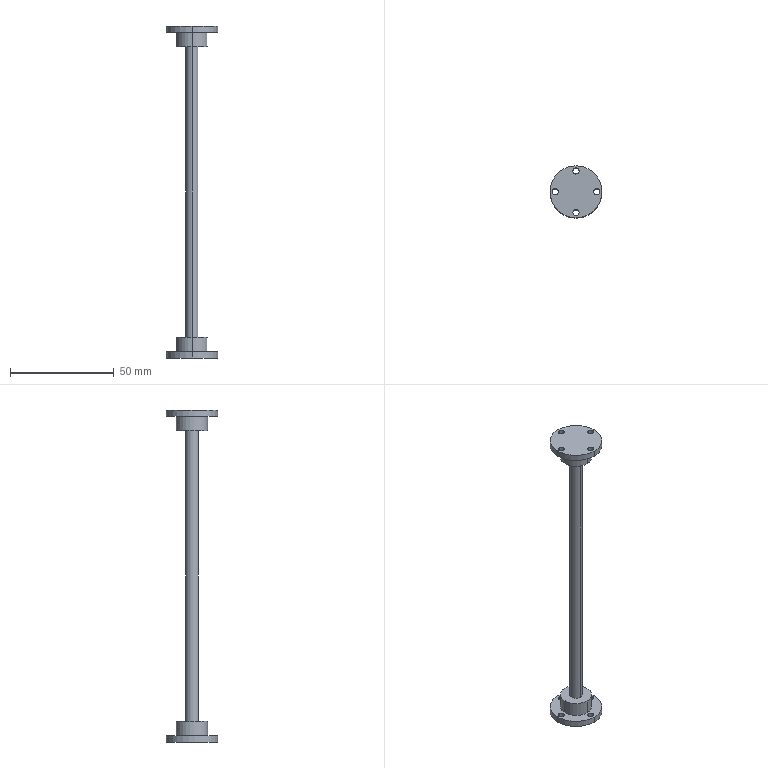Part | SolidWorks | features ICE 1, MirrorPattern 1, Revolution 1 | 1 solid | 32 faces | box 25 x 25 x 160 mm | volume 9208 mm3 | cylinder 26 | plane 6 | commonest cylinder face diameters 3 x16 15 x4 25 x4 6 x2
STEP:
#1=CARTESIAN_POINT('',(-10.,1.5,80.));
#2=VERTEX_POINT('',#1);
#3=CARTESIAN_POINT('',(-10.,-1.5,80.));
#4=VERTEX_POINT('',#3);
#5=CARTESIAN_POINT('',(-10.,0.,80.));
#6=DIRECTION('',(0.,0.,1.));
#7=DIRECTION('',(0.,-1.,0.));
#8=AXIS2_PLACEMENT_3D('',#5,#6,#7);
#9=CIRCLE('',#8,1.5);
#10=EDGE_CURVE('',#2,#4,#9,.T.);
#11=ORIENTED_EDGE('',*,*,#10,.T.);
#12=CARTESIAN_POINT('',(-10.,-1.5,77.));
#13=VERTEX_POINT('',#12);
#14=CARTESIAN_POINT('',(-10.,-1.5,84.));
#15=DIRECTION('',(0.,0.,-1.));
#16=VECTOR('',#15,1000.);
#17=LINE('',#14,#16);
#18=EDGE_CURVE('',#4,#13,#17,.T.);
#19=ORIENTED_EDGE('',*,*,#18,.T.);
#20=CARTESIAN_POINT('',(-10.,1.5,77.));
#21=VERTEX_POINT('',#20);
#22=CARTESIAN_POINT('',(-10.,0.,77.));
#23=DIRECTION('',(0.,0.,-1.));
#24=DIRECTION('',(0.,1.,0.));
#25=AXIS2_PLACEMENT_3D('',#22,#23,#24);
#26=CIRCLE('',#25,1.5);
#27=EDGE_CURVE('',#13,#21,#26,.T.);
#28=ORIENTED_EDGE('',*,*,#27,.T.);
#29=CARTESIAN_POINT('',(-10.,1.5,84.));
#30=DIRECTION('',(0.,0.,-1.));
#31=VECTOR('',#30,1000.);
#32=LINE('',#29,#31);
#33=EDGE_CURVE('',#2,#21,#32,.T.);
#34=ORIENTED_EDGE('',*,*,#33,.F.);
#35=EDGE_LOOP('',(#11,#19,#28,#34));
#36=FACE_OUTER_BOUND('',#35,.T.);
#37=CARTESIAN_POINT('',(-10.,0.,84.));
#38=DIRECTION('',(0.,0.,-1.));
#39=DIRECTION('',(0.,1.,0.));
#40=AXIS2_PLACEMENT_3D('',#37,#38,#39);
#41=CYLINDRICAL_SURFACE('',#40,1.5);
#42=ADVANCED_FACE('',(#36),#41,.F.);
#43=CARTESIAN_POINT('',(0.,-8.5,80.));
#44=VERTEX_POINT('',#43);
#45=CARTESIAN_POINT('',(0.,-11.5,80.));
#46=VERTEX_POINT('',#45);
#47=CARTESIAN_POINT('',(0.,-10.,80.));
#48=DIRECTION('',(0.,0.,1.));
#49=DIRECTION('',(0.,-1.,0.));
#50=AXIS2_PLACEMENT_3D('',#47,#48,#49);
#51=CIRCLE('',#50,1.5);
#52=EDGE_CURVE('',#44,#46,#51,.T.);
#53=ORIENTED_EDGE('',*,*,#52,.T.);
#54=CARTESIAN_POINT('',(0.,-11.5,77.));
#55=VERTEX_POINT('',#54);
#56=CARTESIAN_POINT('',(0.,-11.5,84.));
#57=DIRECTION('',(0.,0.,-1.));
#58=VECTOR('',#57,1000.);
#59=LINE('',#56,#58);
#60=EDGE_CURVE('',#46,#55,#59,.T.);
#61=ORIENTED_EDGE('',*,*,#60,.T.);
#62=CARTESIAN_POINT('',(0.,-8.5,77.));
#63=VERTEX_POINT('',#62);
#64=CARTESIAN_POINT('',(0.,-10.,77.));
#65=DIRECTION('',(0.,0.,-1.));
#66=DIRECTION('',(0.,1.,0.));
#67=AXIS2_PLACEMENT_3D('',#64,#65,#66);
#68=CIRCLE('',#67,1.5);
#69=EDGE_CURVE('',#55,#63,#68,.T.);
#70=ORIENTED_EDGE('',*,*,#69,.T.);
#71=CARTESIAN_POINT('',(0.,-8.5,84.));
#72=DIRECTION('',(0.,0.,-1.));
#73=VECTOR('',#72,1000.);
#74=LINE('',#71,#73);
#75=EDGE_CURVE('',#44,#63,#74,.T.);
#76=ORIENTED_EDGE('',*,*,#75,.F.);
#77=EDGE_LOOP('',(#53,#61,#70,#76));
#78=FACE_OUTER_BOUND('',#77,.T.);
#79=CARTESIAN_POINT('',(0.,-10.,84.));
#80=DIRECTION('',(0.,0.,-1.));
#81=DIRECTION('',(0.,1.,0.));
#82=AXIS2_PLACEMENT_3D('',#79,#80,#81);
#83=CYLINDRICAL_SURFACE('',#82,1.5);
#84=ADVANCED_FACE('',(#78),#83,.F.);
#85=CARTESIAN_POINT('',(10.,1.5,80.));
#86=VERTEX_POINT('',#85);
#87=CARTESIAN_POINT('',(10.,-1.5,80.));
#88=VERTEX_POINT('',#87);
#89=CARTESIAN_POINT('',(10.,0.,80.));
#90=DIRECTION('',(0.,0.,1.));
#91=DIRECTION('',(0.,-1.,0.));
#92=AXIS2_PLACEMENT_3D('',#89,#90,#91);
#93=CIRCLE('',#92,1.5);
#94=EDGE_CURVE('',#86,#88,#93,.T.);
#95=ORIENTED_EDGE('',*,*,#94,.T.);
#96=CARTESIAN_POINT('',(10.,-1.5,77.));
#97=VERTEX_POINT('',#96);
#98=CARTESIAN_POINT('',(10.,-1.5,84.));
#99=DIRECTION('',(0.,0.,-1.));
#100=VECTOR('',#99,1000.);
#101=LINE('',#98,#100);
#102=EDGE_CURVE('',#88,#97,#101,.T.);
#103=ORIENTED_EDGE('',*,*,#102,.T.);
#104=CARTESIAN_POINT('',(10.,1.5,77.));
#105=VERTEX_POINT('',#104);
#106=CARTESIAN_POINT('',(10.,0.,77.));
#107=DIRECTION('',(0.,0.,-1.));
#108=DIRECTION('',(0.,1.,0.));
#109=AXIS2_PLACEMENT_3D('',#106,#107,#108);
#110=CIRCLE('',#109,1.5);
#111=EDGE_CURVE('',#97,#105,#110,.T.);
#112=ORIENTED_EDGE('',*,*,#111,.T.);
#113=CARTESIAN_POINT('',(10.,1.5,84.));
#114=DIRECTION('',(0.,0.,-1.));
#115=VECTOR('',#114,1000.);
#116=LINE('',#113,#115);
#117=EDGE_CURVE('',#86,#105,#116,.T.);
#118=ORIENTED_EDGE('',*,*,#117,.F.);
#119=EDGE_LOOP('',(#95,#103,#112,#118));
#120=FACE_OUTER_BOUND('',#119,.T.);
#121=CARTESIAN_POINT('',(10.,0.,84.));
#122=DIRECTION('',(0.,0.,-1.));
#123=DIRECTION('',(0.,1.,0.));
#124=AXIS2_PLACEMENT_3D('',#121,#122,#123);
#125=CYLINDRICAL_SURFACE('',#124,1.5);
#126=ADVANCED_FACE('',(#120),#125,.F.);
#127=CARTESIAN_POINT('',(0.,11.5,80.));
#128=VERTEX_POINT('',#127);
#129=CARTESIAN_POINT('',(0.,8.5,80.));
#130=VERTEX_POINT('',#129);
#131=CARTESIAN_POINT('',(0.,10.,80.));
#132=DIRECTION('',(0.,0.,1.));
#133=DIRECTION('',(0.,-1.,0.));
#134=AXIS2_PLACEMENT_3D('',#131,#132,#133);
#135=CIRCLE('',#134,1.5);
#136=EDGE_CURVE('',#128,#130,#135,.T.);
#137=ORIENTED_EDGE('',*,*,#136,.T.);
#138=CARTESIAN_POINT('',(0.,8.5,77.));
#139=VERTEX_POINT('',#138);
#140=CARTESIAN_POINT('',(0.,8.5,84.));
#141=DIRECTION('',(0.,0.,-1.));
#142=VECTOR('',#141,1000.);
#143=LINE('',#140,#142);
#144=EDGE_CURVE('',#130,#139,#143,.T.);
#145=ORIENTED_EDGE('',*,*,#144,.T.);
#146=CARTESIAN_POINT('',(0.,11.5,77.));
#147=VERTEX_POINT('',#146);
#148=CARTESIAN_POINT('',(0.,10.,77.));
#149=DIRECTION('',(0.,0.,-1.));
#150=DIRECTION('',(0.,1.,0.));
#151=AXIS2_PLACEMENT_3D('',#148,#149,#150);
#152=CIRCLE('',#151,1.5);
#153=EDGE_CURVE('',#139,#147,#152,.T.);
#154=ORIENTED_EDGE('',*,*,#153,.T.);
#155=CARTESIAN_POINT('',(0.,11.5,84.));
#156=DIRECTION('',(0.,0.,-1.));
#157=VECTOR('',#156,1000.);
#158=LINE('',#155,#157);
#159=EDGE_CURVE('',#128,#147,#158,.T.);
#160=ORIENTED_EDGE('',*,*,#159,.F.);
#161=EDGE_LOOP('',(#137,#145,#154,#160));
#162=FACE_OUTER_BOUND('',#161,.T.);
#163=CARTESIAN_POINT('',(0.,10.,84.));
#164=DIRECTION('',(0.,0.,-1.));
#165=DIRECTION('',(0.,1.,0.));
#166=AXIS2_PLACEMENT_3D('',#163,#164,#165);
#167=CYLINDRICAL_SURFACE('',#166,1.5);
#168=ADVANCED_FACE('',(#162),#167,.F.);
#169=CARTESIAN_POINT('',(-10.,1.5,-77.));
#170=VERTEX_POINT('',#169);
#171=CARTESIAN_POINT('',(-10.,-1.5,-77.));
#172=VERTEX_POINT('',#171);
#173=CARTESIAN_POINT('',(-10.,0.,-77.));
#174=DIRECTION('',(0.,0.,1.));
#175=DIRECTION('',(0.,-1.,0.));
#176=AXIS2_PLACEMENT_3D('',#173,#174,#175);
#177=CIRCLE('',#176,1.5);
#178=EDGE_CURVE('',#170,#172,#177,.T.);
#179=ORIENTED_EDGE('',*,*,#178,.T.);
#180=CARTESIAN_POINT('',(-10.,-1.5,-80.));
#181=VERTEX_POINT('',#180);
#182=CARTESIAN_POINT('',(-10.,-1.5,84.));
#183=DIRECTION('',(0.,0.,-1.));
#184=VECTOR('',#183,1000.);
#185=LINE('',#182,#184);
#186=EDGE_CURVE('',#172,#181,#185,.T.);
#187=ORIENTED_EDGE('',*,*,#186,.T.);
#188=CARTESIAN_POINT('',(-10.,1.5,-80.));
#189=VERTEX_POINT('',#188);
#190=CARTESIAN_POINT('',(-10.,0.,-80.));
#191=DIRECTION('',(0.,0.,-1.));
#192=DIRECTION('',(0.,1.,0.));
#193=AXIS2_PLACEMENT_3D('',#190,#191,#192);
#194=CIRCLE('',#193,1.5);
#195=EDGE_CURVE('',#181,#189,#194,.T.);
#196=ORIENTED_EDGE('',*,*,#195,.T.);
#197=CARTESIAN_POINT('',(-10.,1.5,84.));
#198=DIRECTION('',(0.,0.,-1.));
#199=VECTOR('',#198,1000.);
#200=LINE('',#197,#199);
#201=EDGE_CURVE('',#170,#189,#200,.T.);
#202=ORIENTED_EDGE('',*,*,#201,.F.);
#203=EDGE_LOOP('',(#179,#187,#196,#202));
#204=FACE_OUTER_BOUND('',#203,.T.);
#205=CARTESIAN_POINT('',(-10.,0.,84.));
#206=DIRECTION('',(0.,0.,-1.));
#207=DIRECTION('',(0.,1.,0.));
#208=AXIS2_PLACEMENT_3D('',#205,#206,#207);
#209=CYLINDRICAL_SURFACE('',#208,1.5);
#210=ADVANCED_FACE('',(#204),#209,.F.);
#211=CARTESIAN_POINT('',(0.,-8.5,-77.));
#212=VERTEX_POINT('',#211);
#213=CARTESIAN_POINT('',(0.,-11.5,-77.));
#214=VERTEX_POINT('',#213);
#215=CARTESIAN_POINT('',(0.,-10.,-77.));
#216=DIRECTION('',(0.,0.,1.));
#217=DIRECTION('',(0.,-1.,0.));
#218=AXIS2_PLACEMENT_3D('',#215,#216,#217);
#219=CIRCLE('',#218,1.5);
#220=EDGE_CURVE('',#212,#214,#219,.T.);
#221=ORIENTED_EDGE('',*,*,#220,.T.);
#222=CARTESIAN_POINT('',(0.,-11.5,-80.));
#223=VERTEX_POINT('',#222);
#224=CARTESIAN_POINT('',(0.,-11.5,84.));
#225=DIRECTION('',(0.,0.,-1.));
#226=VECTOR('',#225,1000.);
#227=LINE('',#224,#226);
#228=EDGE_CURVE('',#214,#223,#227,.T.);
#229=ORIENTED_EDGE('',*,*,#228,.T.);
#230=CARTESIAN_POINT('',(0.,-8.5,-80.));
#231=VERTEX_POINT('',#230);
#232=CARTESIAN_POINT('',(0.,-10.,-80.));
#233=DIRECTION('',(0.,0.,-1.));
#234=DIRECTION('',(0.,1.,0.));
#235=AXIS2_PLACEMENT_3D('',#232,#233,#234);
#236=CIRCLE('',#235,1.5);
#237=EDGE_CURVE('',#223,#231,#236,.T.);
#238=ORIENTED_EDGE('',*,*,#237,.T.);
#239=CARTESIAN_POINT('',(0.,-8.5,84.));
#240=DIRECTION('',(0.,0.,-1.));
#241=VECTOR('',#240,1000.);
#242=LINE('',#239,#241);
#243=EDGE_CURVE('',#212,#231,#242,.T.);
#244=ORIENTED_EDGE('',*,*,#243,.F.);
#245=EDGE_LOOP('',(#221,#229,#238,#244));
#246=FACE_OUTER_BOUND('',#245,.T.);
#247=CARTESIAN_POINT('',(0.,-10.,84.));
#248=DIRECTION('',(0.,0.,-1.));
#249=DIRECTION('',(0.,1.,0.));
#250=AXIS2_PLACEMENT_3D('',#247,#248,#249);
#251=CYLINDRICAL_SURFACE('',#250,1.5);
#252=ADVANCED_FACE('',(#246),#251,.F.);
#253=CARTESIAN_POINT('',(10.,1.5,-77.));
#254=VERTEX_POINT('',#253);
#255=CARTESIAN_POINT('',(10.,-1.5,-77.));
#256=VERTEX_POINT('',#255);
#257=CARTESIAN_POINT('',(10.,0.,-77.));
#258=DIRECTION('',(0.,0.,1.));
#259=DIRECTION('',(0.,-1.,0.));
#260=AXIS2_PLACEMENT_3D('',#257,#258,#259);
#261=CIRCLE('',#260,1.5);
#262=EDGE_CURVE('',#254,#256,#261,.T.);
#263=ORIENTED_EDGE('',*,*,#262,.T.);
#264=CARTESIAN_POINT('',(10.,-1.5,-80.));
#265=VERTEX_POINT('',#264);
#266=CARTESIAN_POINT('',(10.,-1.5,84.));
#267=DIRECTION('',(0.,0.,-1.));
#268=VECTOR('',#267,1000.);
#269=LINE('',#266,#268);
#270=EDGE_CURVE('',#256,#265,#269,.T.);
#271=ORIENTED_EDGE('',*,*,#270,.T.);
#272=CARTESIAN_POINT('',(10.,1.5,-80.));
#273=VERTEX_POINT('',#272);
#274=CARTESIAN_POINT('',(10.,0.,-80.));
#275=DIRECTION('',(0.,0.,-1.));
#276=DIRECTION('',(0.,1.,0.));
#277=AXIS2_PLACEMENT_3D('',#274,#275,#276);
#278=CIRCLE('',#277,1.5);
#279=EDGE_CURVE('',#265,#273,#278,.T.);
#280=ORIENTED_EDGE('',*,*,#279,.T.);
#281=CARTESIAN_POINT('',(10.,1.5,84.));
#282=DIRECTION('',(0.,0.,-1.));
#283=VECTOR('',#282,1000.);
#284=LINE('',#281,#283);
#285=EDGE_CURVE('',#254,#273,#284,.T.);
#286=ORIENTED_EDGE('',*,*,#285,.F.);
#287=EDGE_LOOP('',(#263,#271,#280,#286));
#288=FACE_OUTER_BOUND('',#287,.T.);
#289=CARTESIAN_POINT('',(10.,0.,84.));
#290=DIRECTION('',(0.,0.,-1.));
#291=DIRECTION('',(0.,1.,0.));
#292=AXIS2_PLACEMENT_3D('',#289,#290,#291);
#293=CYLINDRICAL_SURFACE('',#292,1.5);
#294=ADVANCED_FACE('',(#288),#293,.F.);
#295=CARTESIAN_POINT('',(0.,11.5,-77.));
#296=VERTEX_POINT('',#295);
#297=CARTESIAN_POINT('',(0.,8.5,-77.));
#298=VERTEX_POINT('',#297);
#299=CARTESIAN_POINT('',(0.,10.,-77.));
#300=DIRECTION('',(0.,0.,1.));
#301=DIRECTION('',(0.,-1.,0.));
#302=AXIS2_PLACEMENT_3D('',#299,#300,#301);
#303=CIRCLE('',#302,1.5);
#304=EDGE_CURVE('',#296,#298,#303,.T.);
#305=ORIENTED_EDGE('',*,*,#304,.T.);
#306=CARTESIAN_POINT('',(0.,8.5,-80.));
#307=VERTEX_POINT('',#306);
#308=CARTESIAN_POINT('',(0.,8.5,84.));
#309=DIRECTION('',(0.,0.,-1.));
#310=VECTOR('',#309,1000.);
#311=LINE('',#308,#310);
#312=EDGE_CURVE('',#298,#307,#311,.T.);
#313=ORIENTED_EDGE('',*,*,#312,.T.);
#314=CARTESIAN_POINT('',(0.,11.5,-80.));
#315=VERTEX_POINT('',#314);
#316=CARTESIAN_POINT('',(0.,10.,-80.));
#317=DIRECTION('',(0.,0.,-1.));
#318=DIRECTION('',(0.,1.,0.));
#319=AXIS2_PLACEMENT_3D('',#316,#317,#318);
#320=CIRCLE('',#319,1.5);
#321=EDGE_CURVE('',#307,#315,#320,.T.);
#322=ORIENTED_EDGE('',*,*,#321,.T.);
#323=CARTESIAN_POINT('',(0.,11.5,84.));
#324=DIRECTION('',(0.,0.,-1.));
#325=VECTOR('',#324,1000.);
#326=LINE('',#323,#325);
#327=EDGE_CURVE('',#296,#315,#326,.T.);
#328=ORIENTED_EDGE('',*,*,#327,.F.);
#329=EDGE_LOOP('',(#305,#313,#322,#328));
#330=FACE_OUTER_BOUND('',#329,.T.);
#331=CARTESIAN_POINT('',(0.,10.,84.));
#332=DIRECTION('',(0.,0.,-1.));
#333=DIRECTION('',(0.,1.,0.));
#334=AXIS2_PLACEMENT_3D('',#331,#332,#333);
#335=CYLINDRICAL_SURFACE('',#334,1.5);
#336=ADVANCED_FACE('',(#330),#335,.F.);
#337=CARTESIAN_POINT('',(0.,-7.5,-77.));
#338=VERTEX_POINT('',#337);
#339=CARTESIAN_POINT('',(0.,7.5,-77.));
#340=VERTEX_POINT('',#339);
#341=CARTESIAN_POINT('',(0.,0.,-77.));
#342=DIRECTION('',(0.,0.,-1.));
#343=DIRECTION('',(0.,1.,0.));
#344=AXIS2_PLACEMENT_3D('',#341,#342,#343);
#345=CIRCLE('',#344,7.5);
#346=EDGE_CURVE('',#338,#340,#345,.T.);
#347=ORIENTED_EDGE('',*,*,#346,.F.);
#348=CARTESIAN_POINT('',(0.,-7.5,-70.));
#349=VERTEX_POINT('',#348);
#350=CARTESIAN_POINT('',(0.,-7.5,0.));
#351=DIRECTION('',(0.,0.,1.));
#352=VECTOR('',#351,1000.);
#353=LINE('',#350,#352);
#354=EDGE_CURVE('',#338,#349,#353,.T.);
#355=ORIENTED_EDGE('',*,*,#354,.T.);
#356=CARTESIAN_POINT('',(0.,7.5,-70.));
#357=VERTEX_POINT('',#356);
#358=CARTESIAN_POINT('',(0.,0.,-70.));
#359=DIRECTION('',(0.,0.,-1.));
#360=DIRECTION('',(0.,1.,0.));
#361=AXIS2_PLACEMENT_3D('',#358,#359,#360);
#362=CIRCLE('',#361,7.5);
#363=EDGE_CURVE('',#349,#357,#362,.T.);
#364=ORIENTED_EDGE('',*,*,#363,.T.);
#365=CARTESIAN_POINT('',(0.,7.5,0.));
#366=DIRECTION('',(0.,0.,1.));
#367=VECTOR('',#366,1000.);
#368=LINE('',#365,#367);
#369=EDGE_CURVE('',#340,#357,#368,.T.);
#370=ORIENTED_EDGE('',*,*,#369,.F.);
#371=EDGE_LOOP('',(#347,#355,#364,#370));
#372=FACE_OUTER_BOUND('',#371,.T.);
#373=CARTESIAN_POINT('',(0.,0.,0.));
#374=DIRECTION('',(0.,0.,1.));
#375=DIRECTION('',(0.,1.,0.));
#376=AXIS2_PLACEMENT_3D('',#373,#374,#375);
#377=CYLINDRICAL_SURFACE('',#376,7.5);
#378=ADVANCED_FACE('',(#372),#377,.T.);
#379=CARTESIAN_POINT('',(0.,-12.5,-80.));
#380=VERTEX_POINT('',#379);
#381=CARTESIAN_POINT('',(0.,12.5,-80.));
#382=VERTEX_POINT('',#381);
#383=CARTESIAN_POINT('',(0.,0.,-80.));
#384=DIRECTION('',(0.,0.,-1.));
#385=DIRECTION('',(0.,1.,0.));
#386=AXIS2_PLACEMENT_3D('',#383,#384,#385);
#387=CIRCLE('',#386,12.5);
#388=EDGE_CURVE('',#380,#382,#387,.T.);
#389=ORIENTED_EDGE('',*,*,#388,.F.);
#390=CARTESIAN_POINT('',(0.,-12.5,-77.));
#391=VERTEX_POINT('',#390);
#392=CARTESIAN_POINT('',(0.,-12.5,0.));
#393=DIRECTION('',(0.,0.,1.));
#394=VECTOR('',#393,1000.);
#395=LINE('',#392,#394);
#396=EDGE_CURVE('',#380,#391,#395,.T.);
#397=ORIENTED_EDGE('',*,*,#396,.T.);
#398=CARTESIAN_POINT('',(0.,12.5,-77.));
#399=VERTEX_POINT('',#398);
#400=CARTESIAN_POINT('',(0.,0.,-77.));
#401=DIRECTION('',(0.,0.,-1.));
#402=DIRECTION('',(0.,1.,0.));
#403=AXIS2_PLACEMENT_3D('',#400,#401,#402);
#404=CIRCLE('',#403,12.5);
#405=EDGE_CURVE('',#391,#399,#404,.T.);
#406=ORIENTED_EDGE('',*,*,#405,.T.);
#407=CARTESIAN_POINT('',(0.,12.5,0.));
#408=DIRECTION('',(0.,0.,1.));
#409=VECTOR('',#408,1000.);
#410=LINE('',#407,#409);
#411=EDGE_CURVE('',#382,#399,#410,.T.);
#412=ORIENTED_EDGE('',*,*,#411,.F.);
#413=EDGE_LOOP('',(#389,#397,#406,#412));
#414=FACE_OUTER_BOUND('',#413,.T.);
#415=CARTESIAN_POINT('',(0.,0.,0.));
#416=DIRECTION('',(0.,0.,1.));
#417=DIRECTION('',(0.,1.,0.));
#418=AXIS2_PLACEMENT_3D('',#415,#416,#417);
#419=CYLINDRICAL_SURFACE('',#418,12.5);
#420=ADVANCED_FACE('',(#414),#419,.T.);
#421=CARTESIAN_POINT('',(0.,3.,70.));
#422=VERTEX_POINT('',#421);
#423=CARTESIAN_POINT('',(0.,-3.,70.));
#424=VERTEX_POINT('',#423);
#425=CARTESIAN_POINT('',(0.,0.,70.));
#426=DIRECTION('',(0.,0.,-1.));
#427=DIRECTION('',(0.,1.,0.));
#428=AXIS2_PLACEMENT_3D('',#425,#426,#427);
#429=CIRCLE('',#428,3.);
#430=EDGE_CURVE('',#422,#424,#429,.T.);
#431=ORIENTED_EDGE('',*,*,#430,.T.);
#432=CARTESIAN_POINT('',(0.,-3.,-70.));
#433=VERTEX_POINT('',#432);
#434=CARTESIAN_POINT('',(0.,-3.,0.));
#435=DIRECTION('',(0.,0.,-1.));
#436=VECTOR('',#435,1000.);
#437=LINE('',#434,#436);
#438=EDGE_CURVE('',#424,#433,#437,.T.);
#439=ORIENTED_EDGE('',*,*,#438,.T.);
#440=CARTESIAN_POINT('',(0.,3.,-70.));
#441=VERTEX_POINT('',#440);
#442=CARTESIAN_POINT('',(0.,0.,-70.));
#443=DIRECTION('',(0.,0.,-1.));
#444=DIRECTION('',(0.,1.,0.));
#445=AXIS2_PLACEMENT_3D('',#442,#443,#444);
#446=CIRCLE('',#445,3.);
#447=EDGE_CURVE('',#441,#433,#446,.T.);
#448=ORIENTED_EDGE('',*,*,#447,.F.);
#449=CARTESIAN_POINT('',(0.,3.,0.));
#450=DIRECTION('',(0.,0.,-1.));
#451=VECTOR('',#450,1000.);
#452=LINE('',#449,#451);
#453=EDGE_CURVE('',#422,#441,#452,.T.);
#454=ORIENTED_EDGE('',*,*,#453,.F.);
#455=EDGE_LOOP('',(#431,#439,#448,#454));
#456=FACE_OUTER_BOUND('',#455,.T.);
#457=CARTESIAN_POINT('',(0.,0.,0.));
#458=DIRECTION('',(0.,0.,-1.));
#459=DIRECTION('',(0.,1.,0.));
#460=AXIS2_PLACEMENT_3D('',#457,#458,#459);
#461=CYLINDRICAL_SURFACE('',#460,3.);
#462=ADVANCED_FACE('',(#456),#461,.T.);
#463=CARTESIAN_POINT('',(0.,7.5,77.));
#464=VERTEX_POINT('',#463);
#465=CARTESIAN_POINT('',(0.,-7.5,77.));
#466=VERTEX_POINT('',#465);
#467=CARTESIAN_POINT('',(0.,0.,77.));
#468=DIRECTION('',(0.,0.,-1.));
#469=DIRECTION('',(0.,1.,0.));
#470=AXIS2_PLACEMENT_3D('',#467,#468,#469);
#471=CIRCLE('',#470,7.5);
#472=EDGE_CURVE('',#464,#466,#471,.T.);
#473=ORIENTED_EDGE('',*,*,#472,.T.);
#474=CARTESIAN_POINT('',(0.,-7.5,70.));
#475=VERTEX_POINT('',#474);
#476=CARTESIAN_POINT('',(0.,-7.5,0.));
#477=DIRECTION('',(0.,0.,-1.));
#478=VECTOR('',#477,1000.);
#479=LINE('',#476,#478);
#480=EDGE_CURVE('',#466,#475,#479,.T.);
#481=ORIENTED_EDGE('',*,*,#480,.T.);
#482=CARTESIAN_POINT('',(0.,7.5,70.));
#483=VERTEX_POINT('',#482);
#484=CARTESIAN_POINT('',(0.,0.,70.));
#485=DIRECTION('',(0.,0.,-1.));
#486=DIRECTION('',(0.,1.,0.));
#487=AXIS2_PLACEMENT_3D('',#484,#485,#486);
#488=CIRCLE('',#487,7.5);
#489=EDGE_CURVE('',#483,#475,#488,.T.);
#490=ORIENTED_EDGE('',*,*,#489,.F.);
#491=CARTESIAN_POINT('',(0.,7.5,0.));
#492=DIRECTION('',(0.,0.,-1.));
#493=VECTOR('',#492,1000.);
#494=LINE('',#491,#493);
#495=EDGE_CURVE('',#464,#483,#494,.T.);
#496=ORIENTED_EDGE('',*,*,#495,.F.);
#497=EDGE_LOOP('',(#473,#481,#490,#496));
#498=FACE_OUTER_BOUND('',#497,.T.);
#499=CARTESIAN_POINT('',(0.,0.,0.));
#500=DIRECTION('',(0.,0.,-1.));
#501=DIRECTION('',(0.,1.,0.));
#502=AXIS2_PLACEMENT_3D('',#499,#500,#501);
#503=CYLINDRICAL_SURFACE('',#502,7.5);
#504=ADVANCED_FACE('',(#498),#503,.T.);
#505=CARTESIAN_POINT('',(0.,12.5,80.));
#506=VERTEX_POINT('',#505);
#507=CARTESIAN_POINT('',(0.,-12.5,80.));
#508=VERTEX_POINT('',#507);
#509=CARTESIAN_POINT('',(0.,0.,80.));
#510=DIRECTION('',(0.,0.,-1.));
#511=DIRECTION('',(0.,1.,0.));
#512=AXIS2_PLACEMENT_3D('',#509,#510,#511);
#513=CIRCLE('',#512,12.5);
#514=EDGE_CURVE('',#506,#508,#513,.T.);
#515=ORIENTED_EDGE('',*,*,#514,.T.);
#516=CARTESIAN_POINT('',(0.,-12.5,77.));
#517=VERTEX_POINT('',#516);
#518=CARTESIAN_POINT('',(0.,-12.5,0.));
#519=DIRECTION('',(0.,0.,-1.));
#520=VECTOR('',#519,1000.);
#521=LINE('',#518,#520);
#522=EDGE_CURVE('',#508,#517,#521,.T.);
#523=ORIENTED_EDGE('',*,*,#522,.T.);
#524=CARTESIAN_POINT('',(0.,12.5,77.));
#525=VERTEX_POINT('',#524);
#526=CARTESIAN_POINT('',(0.,0.,77.));
#527=DIRECTION('',(0.,0.,-1.));
#528=DIRECTION('',(0.,1.,0.));
#529=AXIS2_PLACEMENT_3D('',#526,#527,#528);
#530=CIRCLE('',#529,12.5);
#531=EDGE_CURVE('',#525,#517,#530,.T.);
#532=ORIENTED_EDGE('',*,*,#531,.F.);
#533=CARTESIAN_POINT('',(0.,12.5,0.));
#534=DIRECTION('',(0.,0.,-1.));
#535=VECTOR('',#534,1000.);
#536=LINE('',#533,#535);
#537=EDGE_CURVE('',#506,#525,#536,.T.);
#538=ORIENTED_EDGE('',*,*,#537,.F.);
#539=EDGE_LOOP('',(#515,#523,#532,#538));
#540=FACE_OUTER_BOUND('',#539,.T.);
#541=CARTESIAN_POINT('',(0.,0.,0.));
#542=DIRECTION('',(0.,0.,-1.));
#543=DIRECTION('',(0.,1.,0.));
#544=AXIS2_PLACEMENT_3D('',#541,#542,#543);
#545=CYLINDRICAL_SURFACE('',#544,12.5);
#546=ADVANCED_FACE('',(#540),#545,.T.);
#547=ORIENTED_EDGE('',*,*,#10,.F.);
#548=CARTESIAN_POINT('',(-10.,0.,80.));
#549=DIRECTION('',(0.,0.,1.));
#550=DIRECTION('',(0.,-1.,0.));
#551=AXIS2_PLACEMENT_3D('',#548,#549,#550);
#552=CIRCLE('',#551,1.5);
#553=EDGE_CURVE('',#4,#2,#552,.T.);
#554=ORIENTED_EDGE('',*,*,#553,.F.);
#555=EDGE_LOOP('',(#547,#554));
#556=FACE_BOUND('',#555,.T.);
#557=ORIENTED_EDGE('',*,*,#52,.F.);
#558=CARTESIAN_POINT('',(0.,-10.,80.));
#559=DIRECTION('',(0.,0.,1.));
#560=DIRECTION('',(0.,-1.,0.));
#561=AXIS2_PLACEMENT_3D('',#558,#559,#560);
#562=CIRCLE('',#561,1.5);
#563=EDGE_CURVE('',#46,#44,#562,.T.);
#564=ORIENTED_EDGE('',*,*,#563,.F.);
#565=EDGE_LOOP('',(#557,#564));
#566=FACE_BOUND('',#565,.T.);
#567=ORIENTED_EDGE('',*,*,#94,.F.);
#568=CARTESIAN_POINT('',(10.,0.,80.));
#569=DIRECTION('',(0.,0.,1.));
#570=DIRECTION('',(0.,-1.,0.));
#571=AXIS2_PLACEMENT_3D('',#568,#569,#570);
#572=CIRCLE('',#571,1.5);
#573=EDGE_CURVE('',#88,#86,#572,.T.);
#574=ORIENTED_EDGE('',*,*,#573,.F.);
#575=EDGE_LOOP('',(#567,#574));
#576=FACE_BOUND('',#575,.T.);
#577=ORIENTED_EDGE('',*,*,#136,.F.);
#578=CARTESIAN_POINT('',(0.,10.,80.));
#579=DIRECTION('',(0.,0.,1.));
#580=DIRECTION('',(0.,-1.,0.));
#581=AXIS2_PLACEMENT_3D('',#578,#579,#580);
#582=CIRCLE('',#581,1.5);
#583=EDGE_CURVE('',#130,#128,#582,.T.);
#584=ORIENTED_EDGE('',*,*,#583,.F.);
#585=EDGE_LOOP('',(#577,#584));
#586=FACE_BOUND('',#585,.T.);
#587=ORIENTED_EDGE('',*,*,#514,.F.);
#588=CARTESIAN_POINT('',(0.,0.,80.));
#589=DIRECTION('',(0.,0.,-1.));
#590=DIRECTION('',(0.,1.,0.));
#591=AXIS2_PLACEMENT_3D('',#588,#589,#590);
#592=CIRCLE('',#591,12.5);
#593=EDGE_CURVE('',#508,#506,#592,.T.);
#594=ORIENTED_EDGE('',*,*,#593,.F.);
#595=EDGE_LOOP('',(#587,#594));
#596=FACE_OUTER_BOUND('',#595,.T.);
#597=CARTESIAN_POINT('',(0.,0.,80.));
#598=DIRECTION('',(0.,0.,1.));
#599=DIRECTION('',(0.,-1.,0.));
#600=AXIS2_PLACEMENT_3D('',#597,#598,#599);
#601=PLANE('',#600);
#602=ADVANCED_FACE('',(#556,#566,#576,#586,#596),#601,.T.);
#603=ORIENTED_EDGE('',*,*,#522,.F.);
#604=ORIENTED_EDGE('',*,*,#593,.T.);
#605=ORIENTED_EDGE('',*,*,#537,.T.);
#606=CARTESIAN_POINT('',(0.,0.,77.));
#607=DIRECTION('',(0.,0.,-1.));
#608=DIRECTION('',(0.,1.,0.));
#609=AXIS2_PLACEMENT_3D('',#606,#607,#608);
#610=CIRCLE('',#609,12.5);
#611=EDGE_CURVE('',#517,#525,#610,.T.);
#612=ORIENTED_EDGE('',*,*,#611,.F.);
#613=EDGE_LOOP('',(#603,#604,#605,#612));
#614=FACE_OUTER_BOUND('',#613,.T.);
#615=CARTESIAN_POINT('',(0.,0.,0.));
#616=DIRECTION('',(0.,0.,-1.));
#617=DIRECTION('',(0.,1.,0.));
#618=AXIS2_PLACEMENT_3D('',#615,#616,#617);
#619=CYLINDRICAL_SURFACE('',#618,12.5);
#620=ADVANCED_FACE('',(#614),#619,.T.);
#621=CARTESIAN_POINT('',(-10.,0.,77.));
#622=DIRECTION('',(0.,0.,-1.));
#623=DIRECTION('',(0.,1.,0.));
#624=AXIS2_PLACEMENT_3D('',#621,#622,#623);
#625=CIRCLE('',#624,1.5);
#626=EDGE_CURVE('',#21,#13,#625,.T.);
#627=ORIENTED_EDGE('',*,*,#626,.F.);
#628=ORIENTED_EDGE('',*,*,#27,.F.);
#629=EDGE_LOOP('',(#627,#628));
#630=FACE_BOUND('',#629,.T.);
#631=CARTESIAN_POINT('',(0.,-10.,77.));
#632=DIRECTION('',(0.,0.,-1.));
#633=DIRECTION('',(0.,1.,0.));
#634=AXIS2_PLACEMENT_3D('',#631,#632,#633);
#635=CIRCLE('',#634,1.5);
#636=EDGE_CURVE('',#63,#55,#635,.T.);
#637=ORIENTED_EDGE('',*,*,#636,.F.);
#638=ORIENTED_EDGE('',*,*,#69,.F.);
#639=EDGE_LOOP('',(#637,#638));
#640=FACE_BOUND('',#639,.T.);
#641=CARTESIAN_POINT('',(10.,0.,77.));
#642=DIRECTION('',(0.,0.,-1.));
#643=DIRECTION('',(0.,1.,0.));
#644=AXIS2_PLACEMENT_3D('',#641,#642,#643);
#645=CIRCLE('',#644,1.5);
#646=EDGE_CURVE('',#105,#97,#645,.T.);
#647=ORIENTED_EDGE('',*,*,#646,.F.);
#648=ORIENTED_EDGE('',*,*,#111,.F.);
#649=EDGE_LOOP('',(#647,#648));
#650=FACE_BOUND('',#649,.T.);
#651=CARTESIAN_POINT('',(0.,10.,77.));
#652=DIRECTION('',(0.,0.,-1.));
#653=DIRECTION('',(0.,1.,0.));
#654=AXIS2_PLACEMENT_3D('',#651,#652,#653);
#655=CIRCLE('',#654,1.5);
#656=EDGE_CURVE('',#147,#139,#655,.T.);
#657=ORIENTED_EDGE('',*,*,#656,.F.);
#658=ORIENTED_EDGE('',*,*,#153,.F.);
#659=EDGE_LOOP('',(#657,#658));
#660=FACE_BOUND('',#659,.T.);
#661=ORIENTED_EDGE('',*,*,#531,.T.);
#662=ORIENTED_EDGE('',*,*,#611,.T.);
#663=EDGE_LOOP('',(#661,#662));
#664=FACE_OUTER_BOUND('',#663,.T.);
#665=ORIENTED_EDGE('',*,*,#472,.F.);
#666=CARTESIAN_POINT('',(0.,0.,77.));
#667=DIRECTION('',(0.,0.,-1.));
#668=DIRECTION('',(0.,1.,0.));
#669=AXIS2_PLACEMENT_3D('',#666,#667,#668);
#670=CIRCLE('',#669,7.5);
#671=EDGE_CURVE('',#466,#464,#670,.T.);
#672=ORIENTED_EDGE('',*,*,#671,.F.);
#673=EDGE_LOOP('',(#665,#672));
#674=FACE_BOUND('',#673,.T.);
#675=CARTESIAN_POINT('',(0.,12.5,77.));
#676=DIRECTION('',(0.,0.,-1.));
#677=DIRECTION('',(0.,1.,0.));
#678=AXIS2_PLACEMENT_3D('',#675,#676,#677);
#679=PLANE('',#678);
#680=ADVANCED_FACE('',(#630,#640,#650,#660,#664,#674),#679,.T.);
#681=ORIENTED_EDGE('',*,*,#480,.F.);
#682=ORIENTED_EDGE('',*,*,#671,.T.);
#683=ORIENTED_EDGE('',*,*,#495,.T.);
#684=CARTESIAN_POINT('',(0.,0.,70.));
#685=DIRECTION('',(0.,0.,-1.));
#686=DIRECTION('',(0.,1.,0.));
#687=AXIS2_PLACEMENT_3D('',#684,#685,#686);
#688=CIRCLE('',#687,7.5);
#689=EDGE_CURVE('',#475,#483,#688,.T.);
#690=ORIENTED_EDGE('',*,*,#689,.F.);
#691=EDGE_LOOP('',(#681,#682,#683,#690));
#692=FACE_OUTER_BOUND('',#691,.T.);
#693=CARTESIAN_POINT('',(0.,0.,0.));
#694=DIRECTION('',(0.,0.,-1.));
#695=DIRECTION('',(0.,1.,0.));
#696=AXIS2_PLACEMENT_3D('',#693,#694,#695);
#697=CYLINDRICAL_SURFACE('',#696,7.5);
#698=ADVANCED_FACE('',(#692),#697,.T.);
#699=ORIENTED_EDGE('',*,*,#489,.T.);
#700=ORIENTED_EDGE('',*,*,#689,.T.);
#701=EDGE_LOOP('',(#699,#700));
#702=FACE_OUTER_BOUND('',#701,.T.);
#703=ORIENTED_EDGE('',*,*,#430,.F.);
#704=CARTESIAN_POINT('',(0.,0.,70.));
#705=DIRECTION('',(0.,0.,-1.));
#706=DIRECTION('',(0.,1.,0.));
#707=AXIS2_PLACEMENT_3D('',#704,#705,#706);
#708=CIRCLE('',#707,3.);
#709=EDGE_CURVE('',#424,#422,#708,.T.);
#710=ORIENTED_EDGE('',*,*,#709,.F.);
#711=EDGE_LOOP('',(#703,#710));
#712=FACE_BOUND('',#711,.T.);
#713=CARTESIAN_POINT('',(0.,7.5,70.));
#714=DIRECTION('',(0.,0.,-1.));
#715=DIRECTION('',(0.,1.,0.));
#716=AXIS2_PLACEMENT_3D('',#713,#714,#715);
#717=PLANE('',#716);
#718=ADVANCED_FACE('',(#702,#712),#717,.T.);
#719=ORIENTED_EDGE('',*,*,#438,.F.);
#720=ORIENTED_EDGE('',*,*,#709,.T.);
#721=ORIENTED_EDGE('',*,*,#453,.T.);
#722=CARTESIAN_POINT('',(0.,0.,-70.));
#723=DIRECTION('',(0.,0.,-1.));
#724=DIRECTION('',(0.,1.,0.));
#725=AXIS2_PLACEMENT_3D('',#722,#723,#724);
#726=CIRCLE('',#725,3.);
#727=EDGE_CURVE('',#433,#441,#726,.T.);
#728=ORIENTED_EDGE('',*,*,#727,.F.);
#729=EDGE_LOOP('',(#719,#720,#721,#728));
#730=FACE_OUTER_BOUND('',#729,.T.);
#731=CARTESIAN_POINT('',(0.,0.,0.));
#732=DIRECTION('',(0.,0.,-1.));
#733=DIRECTION('',(0.,1.,0.));
#734=AXIS2_PLACEMENT_3D('',#731,#732,#733);
#735=CYLINDRICAL_SURFACE('',#734,3.);
#736=ADVANCED_FACE('',(#730),#735,.T.);
#737=CARTESIAN_POINT('',(-10.,0.,-80.));
#738=DIRECTION('',(0.,0.,-1.));
#739=DIRECTION('',(0.,1.,0.));
#740=AXIS2_PLACEMENT_3D('',#737,#738,#739);
#741=CIRCLE('',#740,1.5);
#742=EDGE_CURVE('',#189,#181,#741,.T.);
#743=ORIENTED_EDGE('',*,*,#742,.F.);
#744=ORIENTED_EDGE('',*,*,#195,.F.);
#745=EDGE_LOOP('',(#743,#744));
#746=FACE_BOUND('',#745,.T.);
#747=CARTESIAN_POINT('',(0.,-10.,-80.));
#748=DIRECTION('',(0.,0.,-1.));
#749=DIRECTION('',(0.,1.,0.));
#750=AXIS2_PLACEMENT_3D('',#747,#748,#749);
#751=CIRCLE('',#750,1.5);
#752=EDGE_CURVE('',#231,#223,#751,.T.);
#753=ORIENTED_EDGE('',*,*,#752,.F.);
#754=ORIENTED_EDGE('',*,*,#237,.F.);
#755=EDGE_LOOP('',(#753,#754));
#756=FACE_BOUND('',#755,.T.);
#757=CARTESIAN_POINT('',(10.,0.,-80.));
#758=DIRECTION('',(0.,0.,-1.));
#759=DIRECTION('',(0.,1.,0.));
#760=AXIS2_PLACEMENT_3D('',#757,#758,#759);
#761=CIRCLE('',#760,1.5);
#762=EDGE_CURVE('',#273,#265,#761,.T.);
#763=ORIENTED_EDGE('',*,*,#762,.F.);
#764=ORIENTED_EDGE('',*,*,#279,.F.);
#765=EDGE_LOOP('',(#763,#764));
#766=FACE_BOUND('',#765,.T.);
#767=CARTESIAN_POINT('',(0.,10.,-80.));
#768=DIRECTION('',(0.,0.,-1.));
#769=DIRECTION('',(0.,1.,0.));
#770=AXIS2_PLACEMENT_3D('',#767,#768,#769);
#771=CIRCLE('',#770,1.5);
#772=EDGE_CURVE('',#315,#307,#771,.T.);
#773=ORIENTED_EDGE('',*,*,#772,.F.);
#774=ORIENTED_EDGE('',*,*,#321,.F.);
#775=EDGE_LOOP('',(#773,#774));
#776=FACE_BOUND('',#775,.T.);
#777=CARTESIAN_POINT('',(0.,0.,-80.));
#778=DIRECTION('',(0.,0.,-1.));
#779=DIRECTION('',(0.,1.,0.));
#780=AXIS2_PLACEMENT_3D('',#777,#778,#779);
#781=CIRCLE('',#780,12.5);
#782=EDGE_CURVE('',#382,#380,#781,.T.);
#783=ORIENTED_EDGE('',*,*,#782,.T.);
#784=ORIENTED_EDGE('',*,*,#388,.T.);
#785=EDGE_LOOP('',(#783,#784));
#786=FACE_OUTER_BOUND('',#785,.T.);
#787=CARTESIAN_POINT('',(0.,0.,-80.));
#788=DIRECTION('',(0.,0.,-1.));
#789=DIRECTION('',(0.,-1.,0.));
#790=AXIS2_PLACEMENT_3D('',#787,#788,#789);
#791=PLANE('',#790);
#792=ADVANCED_FACE('',(#746,#756,#766,#776,#786),#791,.T.);
#793=ORIENTED_EDGE('',*,*,#396,.F.);
#794=ORIENTED_EDGE('',*,*,#782,.F.);
#795=ORIENTED_EDGE('',*,*,#411,.T.);
#796=CARTESIAN_POINT('',(0.,0.,-77.));
#797=DIRECTION('',(0.,0.,-1.));
#798=DIRECTION('',(0.,1.,0.));
#799=AXIS2_PLACEMENT_3D('',#796,#797,#798);
#800=CIRCLE('',#799,12.5);
#801=EDGE_CURVE('',#399,#391,#800,.T.);
#802=ORIENTED_EDGE('',*,*,#801,.T.);
#803=EDGE_LOOP('',(#793,#794,#795,#802));
#804=FACE_OUTER_BOUND('',#803,.T.);
#805=CARTESIAN_POINT('',(0.,0.,0.));
#806=DIRECTION('',(0.,0.,1.));
#807=DIRECTION('',(0.,1.,0.));
#808=AXIS2_PLACEMENT_3D('',#805,#806,#807);
#809=CYLINDRICAL_SURFACE('',#808,12.5);
#810=ADVANCED_FACE('',(#804),#809,.T.);
#811=ORIENTED_EDGE('',*,*,#178,.F.);
#812=CARTESIAN_POINT('',(-10.,0.,-77.));
#813=DIRECTION('',(0.,0.,1.));
#814=DIRECTION('',(0.,-1.,0.));
#815=AXIS2_PLACEMENT_3D('',#812,#813,#814);
#816=CIRCLE('',#815,1.5);
#817=EDGE_CURVE('',#172,#170,#816,.T.);
#818=ORIENTED_EDGE('',*,*,#817,.F.);
#819=EDGE_LOOP('',(#811,#818));
#820=FACE_BOUND('',#819,.T.);
#821=ORIENTED_EDGE('',*,*,#220,.F.);
#822=CARTESIAN_POINT('',(0.,-10.,-77.));
#823=DIRECTION('',(0.,0.,1.));
#824=DIRECTION('',(0.,-1.,0.));
#825=AXIS2_PLACEMENT_3D('',#822,#823,#824);
#826=CIRCLE('',#825,1.5);
#827=EDGE_CURVE('',#214,#212,#826,.T.);
#828=ORIENTED_EDGE('',*,*,#827,.F.);
#829=EDGE_LOOP('',(#821,#828));
#830=FACE_BOUND('',#829,.T.);
#831=ORIENTED_EDGE('',*,*,#262,.F.);
#832=CARTESIAN_POINT('',(10.,0.,-77.));
#833=DIRECTION('',(0.,0.,1.));
#834=DIRECTION('',(0.,-1.,0.));
#835=AXIS2_PLACEMENT_3D('',#832,#833,#834);
#836=CIRCLE('',#835,1.5);
#837=EDGE_CURVE('',#256,#254,#836,.T.);
#838=ORIENTED_EDGE('',*,*,#837,.F.);
#839=EDGE_LOOP('',(#831,#838));
#840=FACE_BOUND('',#839,.T.);
#841=ORIENTED_EDGE('',*,*,#304,.F.);
#842=CARTESIAN_POINT('',(0.,10.,-77.));
#843=DIRECTION('',(0.,0.,1.));
#844=DIRECTION('',(0.,-1.,0.));
#845=AXIS2_PLACEMENT_3D('',#842,#843,#844);
#846=CIRCLE('',#845,1.5);
#847=EDGE_CURVE('',#298,#296,#846,.T.);
#848=ORIENTED_EDGE('',*,*,#847,.F.);
#849=EDGE_LOOP('',(#841,#848));
#850=FACE_BOUND('',#849,.T.);
#851=ORIENTED_EDGE('',*,*,#801,.F.);
#852=ORIENTED_EDGE('',*,*,#405,.F.);
#853=EDGE_LOOP('',(#851,#852));
#854=FACE_OUTER_BOUND('',#853,.T.);
#855=CARTESIAN_POINT('',(0.,0.,-77.));
#856=DIRECTION('',(0.,0.,-1.));
#857=DIRECTION('',(0.,1.,0.));
#858=AXIS2_PLACEMENT_3D('',#855,#856,#857);
#859=CIRCLE('',#858,7.5);
#860=EDGE_CURVE('',#340,#338,#859,.T.);
#861=ORIENTED_EDGE('',*,*,#860,.T.);
#862=ORIENTED_EDGE('',*,*,#346,.T.);
#863=EDGE_LOOP('',(#861,#862));
#864=FACE_BOUND('',#863,.T.);
#865=CARTESIAN_POINT('',(0.,12.5,-77.));
#866=DIRECTION('',(0.,0.,1.));
#867=DIRECTION('',(0.,1.,0.));
#868=AXIS2_PLACEMENT_3D('',#865,#866,#867);
#869=PLANE('',#868);
#870=ADVANCED_FACE('',(#820,#830,#840,#850,#854,#864),#869,.T.);
#871=ORIENTED_EDGE('',*,*,#354,.F.);
#872=ORIENTED_EDGE('',*,*,#860,.F.);
#873=ORIENTED_EDGE('',*,*,#369,.T.);
#874=CARTESIAN_POINT('',(0.,0.,-70.));
#875=DIRECTION('',(0.,0.,-1.));
#876=DIRECTION('',(0.,1.,0.));
#877=AXIS2_PLACEMENT_3D('',#874,#875,#876);
#878=CIRCLE('',#877,7.5);
#879=EDGE_CURVE('',#357,#349,#878,.T.);
#880=ORIENTED_EDGE('',*,*,#879,.T.);
#881=EDGE_LOOP('',(#871,#872,#873,#880));
#882=FACE_OUTER_BOUND('',#881,.T.);
#883=CARTESIAN_POINT('',(0.,0.,0.));
#884=DIRECTION('',(0.,0.,1.));
#885=DIRECTION('',(0.,1.,0.));
#886=AXIS2_PLACEMENT_3D('',#883,#884,#885);
#887=CYLINDRICAL_SURFACE('',#886,7.5);
#888=ADVANCED_FACE('',(#882),#887,.T.);
#889=ORIENTED_EDGE('',*,*,#879,.F.);
#890=ORIENTED_EDGE('',*,*,#363,.F.);
#891=EDGE_LOOP('',(#889,#890));
#892=FACE_OUTER_BOUND('',#891,.T.);
#893=ORIENTED_EDGE('',*,*,#447,.T.);
#894=ORIENTED_EDGE('',*,*,#727,.T.);
#895=EDGE_LOOP('',(#893,#894));
#896=FACE_BOUND('',#895,.T.);
#897=CARTESIAN_POINT('',(0.,7.5,-70.));
#898=DIRECTION('',(0.,0.,1.));
#899=DIRECTION('',(0.,1.,0.));
#900=AXIS2_PLACEMENT_3D('',#897,#898,#899);
#901=PLANE('',#900);
#902=ADVANCED_FACE('',(#892,#896),#901,.T.);
#903=ORIENTED_EDGE('',*,*,#312,.F.);
#904=ORIENTED_EDGE('',*,*,#847,.T.);
#905=ORIENTED_EDGE('',*,*,#327,.T.);
#906=ORIENTED_EDGE('',*,*,#772,.T.);
#907=EDGE_LOOP('',(#903,#904,#905,#906));
#908=FACE_OUTER_BOUND('',#907,.T.);
#909=CARTESIAN_POINT('',(0.,10.,84.));
#910=DIRECTION('',(0.,0.,-1.));
#911=DIRECTION('',(0.,1.,0.));
#912=AXIS2_PLACEMENT_3D('',#909,#910,#911);
#913=CYLINDRICAL_SURFACE('',#912,1.5);
#914=ADVANCED_FACE('',(#908),#913,.F.);
#915=ORIENTED_EDGE('',*,*,#270,.F.);
#916=ORIENTED_EDGE('',*,*,#837,.T.);
#917=ORIENTED_EDGE('',*,*,#285,.T.);
#918=ORIENTED_EDGE('',*,*,#762,.T.);
#919=EDGE_LOOP('',(#915,#916,#917,#918));
#920=FACE_OUTER_BOUND('',#919,.T.);
#921=CARTESIAN_POINT('',(10.,0.,84.));
#922=DIRECTION('',(0.,0.,-1.));
#923=DIRECTION('',(0.,1.,0.));
#924=AXIS2_PLACEMENT_3D('',#921,#922,#923);
#925=CYLINDRICAL_SURFACE('',#924,1.5);
#926=ADVANCED_FACE('',(#920),#925,.F.);
#927=ORIENTED_EDGE('',*,*,#228,.F.);
#928=ORIENTED_EDGE('',*,*,#827,.T.);
#929=ORIENTED_EDGE('',*,*,#243,.T.);
#930=ORIENTED_EDGE('',*,*,#752,.T.);
#931=EDGE_LOOP('',(#927,#928,#929,#930));
#932=FACE_OUTER_BOUND('',#931,.T.);
#933=CARTESIAN_POINT('',(0.,-10.,84.));
#934=DIRECTION('',(0.,0.,-1.));
#935=DIRECTION('',(0.,1.,0.));
#936=AXIS2_PLACEMENT_3D('',#933,#934,#935);
#937=CYLINDRICAL_SURFACE('',#936,1.5);
#938=ADVANCED_FACE('',(#932),#937,.F.);
#939=ORIENTED_EDGE('',*,*,#186,.F.);
#940=ORIENTED_EDGE('',*,*,#817,.T.);
#941=ORIENTED_EDGE('',*,*,#201,.T.);
#942=ORIENTED_EDGE('',*,*,#742,.T.);
#943=EDGE_LOOP('',(#939,#940,#941,#942));
#944=FACE_OUTER_BOUND('',#943,.T.);
#945=CARTESIAN_POINT('',(-10.,0.,84.));
#946=DIRECTION('',(0.,0.,-1.));
#947=DIRECTION('',(0.,1.,0.));
#948=AXIS2_PLACEMENT_3D('',#945,#946,#947);
#949=CYLINDRICAL_SURFACE('',#948,1.5);
#950=ADVANCED_FACE('',(#944),#949,.F.);
#951=ORIENTED_EDGE('',*,*,#144,.F.);
#952=ORIENTED_EDGE('',*,*,#583,.T.);
#953=ORIENTED_EDGE('',*,*,#159,.T.);
#954=ORIENTED_EDGE('',*,*,#656,.T.);
#955=EDGE_LOOP('',(#951,#952,#953,#954));
#956=FACE_OUTER_BOUND('',#955,.T.);
#957=CARTESIAN_POINT('',(0.,10.,84.));
#958=DIRECTION('',(0.,0.,-1.));
#959=DIRECTION('',(0.,1.,0.));
#960=AXIS2_PLACEMENT_3D('',#957,#958,#959);
#961=CYLINDRICAL_SURFACE('',#960,1.5);
#962=ADVANCED_FACE('',(#956),#961,.F.);
#963=ORIENTED_EDGE('',*,*,#102,.F.);
#964=ORIENTED_EDGE('',*,*,#573,.T.);
#965=ORIENTED_EDGE('',*,*,#117,.T.);
#966=ORIENTED_EDGE('',*,*,#646,.T.);
#967=EDGE_LOOP('',(#963,#964,#965,#966));
#968=FACE_OUTER_BOUND('',#967,.T.);
#969=CARTESIAN_POINT('',(10.,0.,84.));
#970=DIRECTION('',(0.,0.,-1.));
#971=DIRECTION('',(0.,1.,0.));
#972=AXIS2_PLACEMENT_3D('',#969,#970,#971);
#973=CYLINDRICAL_SURFACE('',#972,1.5);
#974=ADVANCED_FACE('',(#968),#973,.F.);
#975=ORIENTED_EDGE('',*,*,#60,.F.);
#976=ORIENTED_EDGE('',*,*,#563,.T.);
#977=ORIENTED_EDGE('',*,*,#75,.T.);
#978=ORIENTED_EDGE('',*,*,#636,.T.);
#979=EDGE_LOOP('',(#975,#976,#977,#978));
#980=FACE_OUTER_BOUND('',#979,.T.);
#981=CARTESIAN_POINT('',(0.,-10.,84.));
#982=DIRECTION('',(0.,0.,-1.));
#983=DIRECTION('',(0.,1.,0.));
#984=AXIS2_PLACEMENT_3D('',#981,#982,#983);
#985=CYLINDRICAL_SURFACE('',#984,1.5);
#986=ADVANCED_FACE('',(#980),#985,.F.);
#987=ORIENTED_EDGE('',*,*,#18,.F.);
#988=ORIENTED_EDGE('',*,*,#553,.T.);
#989=ORIENTED_EDGE('',*,*,#33,.T.);
#990=ORIENTED_EDGE('',*,*,#626,.T.);
#991=EDGE_LOOP('',(#987,#988,#989,#990));
#992=FACE_OUTER_BOUND('',#991,.T.);
#993=CARTESIAN_POINT('',(-10.,0.,84.));
#994=DIRECTION('',(0.,0.,-1.));
#995=DIRECTION('',(0.,1.,0.));
#996=AXIS2_PLACEMENT_3D('',#993,#994,#995);
#997=CYLINDRICAL_SURFACE('',#996,1.5);
#998=ADVANCED_FACE('',(#992),#997,.F.);
#999=CLOSED_SHELL('',(#42,#84,#126,#168,#210,#252,#294,#336,#378,#420,#462,#504,#546,#602,#620,#680,#698,#718,#736,#792,#810,#870,#888,#902,#914,#926,#938,#950,#962,#974,#986,#998));
#1000=MANIFOLD_SOLID_BREP('',#999);
#1001=CARTESIAN_POINT('',(0.,0.,0.));
#1002=DIRECTION('',(0.,0.,1.));
#1003=DIRECTION('',(1.,0.,0.));
#1004=AXIS2_PLACEMENT_3D('',#1001,#1002,#1003);
#1005=(LENGTH_UNIT()NAMED_UNIT(*)SI_UNIT(.MILLI.,.METRE.));
#1006=UNCERTAINTY_MEASURE_WITH_UNIT(LENGTH_MEASURE(0.00001),#1005,'','');
#1007=(NAMED_UNIT(*)PLANE_ANGLE_UNIT()SI_UNIT($,.RADIAN.));
#1008=(NAMED_UNIT(*)SI_UNIT($,.STERADIAN.)SOLID_ANGLE_UNIT());
#1009=(GEOMETRIC_REPRESENTATION_CONTEXT(3)GLOBAL_UNCERTAINTY_ASSIGNED_CONTEXT((#1006))GLOBAL_UNIT_ASSIGNED_CONTEXT((#1005,#1007,#1008))REPRESENTATION_CONTEXT('',''));
#1010=ADVANCED_BREP_SHAPE_REPRESENTATION('',(#1000,#1004),#1009);